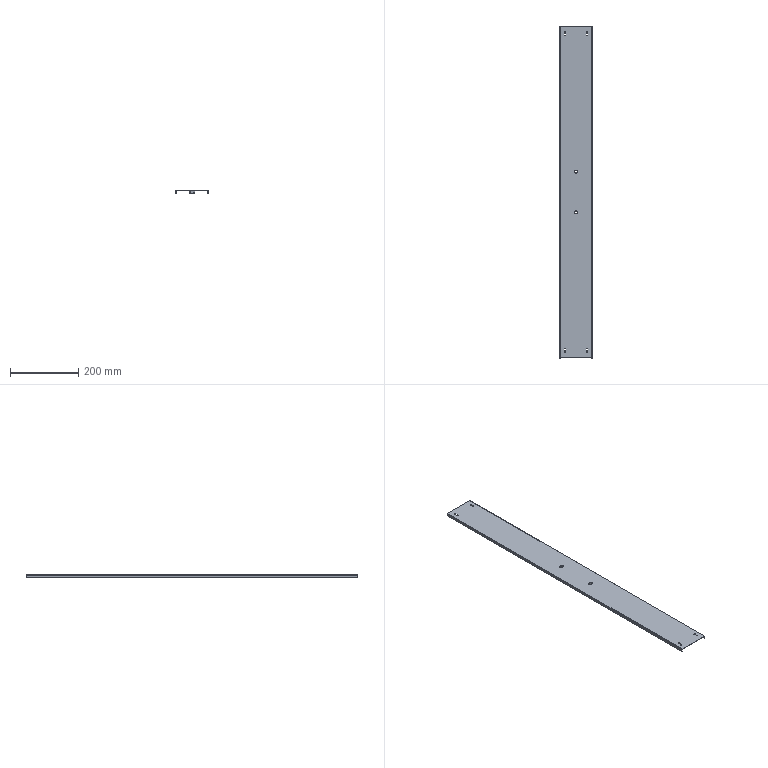Part | SolidWorks | features BaseBody 1 | 1 solid | 62 faces | box 95 x 975 x 8 mm | volume 106450 mm3 | plane 42 | cylinder 20 | commonest cylinder face diameters 5 x8 8 x4 9 x4 0.4 x2 2.4 x2